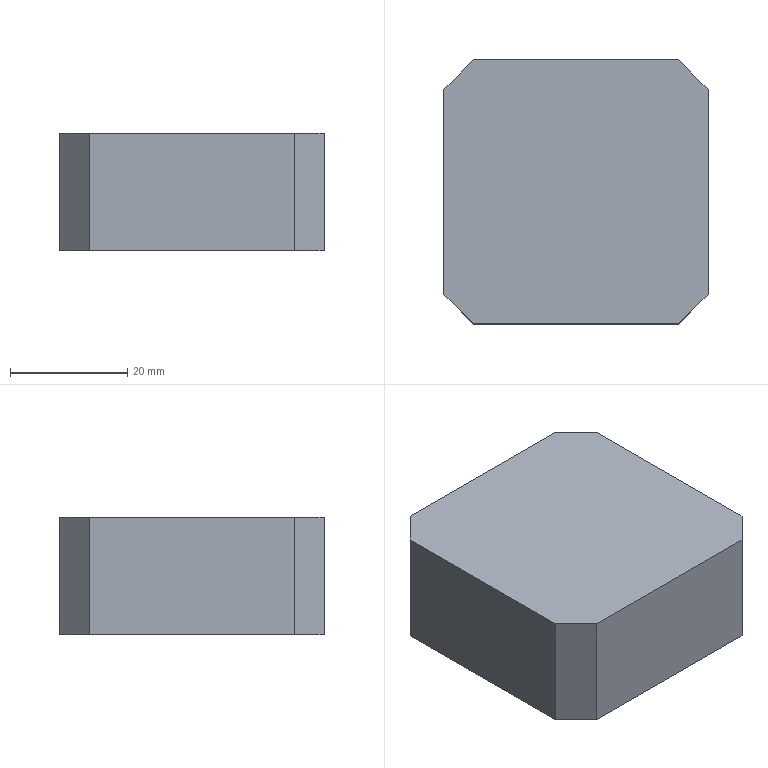Part | STEP file | 2012-06-08-019 | 1 solid | 10 faces | box 45 x 45 x 20 mm | volume 39500 mm3 | plane 10
STEP:
#1=CARTESIAN_POINT('',(0.,0.,0.));
#2=DIRECTION('',(0.,0.,1.));
#3=DIRECTION('',(1.,0.,0.));
#4=AXIS2_PLACEMENT_3D('',#1,#2,#3);
#5=CARTESIAN_POINT('',(22.5,-17.5,20.));
#6=VERTEX_POINT('',#5);
#7=CARTESIAN_POINT('',(22.5,17.5,20.));
#8=VERTEX_POINT('',#7);
#9=CARTESIAN_POINT('',(22.5,22.5,20.));
#10=DIRECTION('',(0.,1.,0.));
#11=VECTOR('',#10,1.);
#12=LINE('',#9,#11);
#13=CARTESIAN_POINT('',(22.5,22.5,20.));
#14=DIRECTION('',(-1.,0.,0.));
#15=DIRECTION('',(0.,-1.,0.));
#16=AXIS2_PLACEMENT_3D('',#13,#14,#15);
#17=PLANE('',#16);
#18=CARTESIAN_POINT('',(0.,0.));
#19=DIRECTION('',(-1.,0.));
#20=VECTOR('',#19,1.);
#21=LINE('',#18,#20);
#22=(GEOMETRIC_REPRESENTATION_CONTEXT(2)PARAMETRIC_REPRESENTATION_CONTEXT()REPRESENTATION_CONTEXT('',''));
#23=DEFINITIONAL_REPRESENTATION('',(#21),#22);
#24=PCURVE('',#17,#23);
#25=CARTESIAN_POINT('',(22.5,-22.5,20.));
#26=DIRECTION('',(0.,0.,1.));
#27=DIRECTION('',(1.,0.,0.));
#28=AXIS2_PLACEMENT_3D('',#25,#26,#27);
#29=PLANE('',#28);
#30=CARTESIAN_POINT('',(0.,45.));
#31=DIRECTION('',(0.,1.));
#32=VECTOR('',#31,1.);
#33=LINE('',#30,#32);
#34=(GEOMETRIC_REPRESENTATION_CONTEXT(2)PARAMETRIC_REPRESENTATION_CONTEXT()REPRESENTATION_CONTEXT('',''));
#35=DEFINITIONAL_REPRESENTATION('',(#33),#34);
#36=PCURVE('',#29,#35);
#37=SURFACE_CURVE('',#12,(#24,#36),.PCURVE_S1.);
#38=EDGE_CURVE('',#6,#8,#37,.T.);
#39=ORIENTED_EDGE('',*,*,#38,.F.);
#40=CARTESIAN_POINT('',(22.5,-17.5,0.));
#41=VERTEX_POINT('',#40);
#42=CARTESIAN_POINT('',(22.5,-17.5,20.));
#43=DIRECTION('',(0.,0.,-1.));
#44=VECTOR('',#43,1.);
#45=LINE('',#42,#44);
#46=CARTESIAN_POINT('',(40.,0.));
#47=DIRECTION('',(0.,-1.));
#48=VECTOR('',#47,1.);
#49=LINE('',#46,#48);
#50=(GEOMETRIC_REPRESENTATION_CONTEXT(2)PARAMETRIC_REPRESENTATION_CONTEXT()REPRESENTATION_CONTEXT('',''));
#51=DEFINITIONAL_REPRESENTATION('',(#49),#50);
#52=PCURVE('',#17,#51);
#53=CARTESIAN_POINT('',(22.5,-17.5,20.));
#54=DIRECTION('',(-0.7071,0.7071,0.));
#55=DIRECTION('',(-0.7071,-0.7071,0.));
#56=AXIS2_PLACEMENT_3D('',#53,#54,#55);
#57=PLANE('',#56);
#58=CARTESIAN_POINT('',(0.,0.));
#59=DIRECTION('',(0.,-1.));
#60=VECTOR('',#59,1.);
#61=LINE('',#58,#60);
#62=(GEOMETRIC_REPRESENTATION_CONTEXT(2)PARAMETRIC_REPRESENTATION_CONTEXT()REPRESENTATION_CONTEXT('',''));
#63=DEFINITIONAL_REPRESENTATION('',(#61),#62);
#64=PCURVE('',#57,#63);
#65=SURFACE_CURVE('',#45,(#52,#64),.PCURVE_S1.);
#66=EDGE_CURVE('',#6,#41,#65,.T.);
#67=ORIENTED_EDGE('',*,*,#66,.T.);
#68=CARTESIAN_POINT('',(22.5,17.5,0.));
#69=VERTEX_POINT('',#68);
#70=CARTESIAN_POINT('',(22.5,22.5,0.));
#71=DIRECTION('',(0.,1.,0.));
#72=VECTOR('',#71,1.);
#73=LINE('',#70,#72);
#74=CARTESIAN_POINT('',(0.,-20.));
#75=DIRECTION('',(-1.,0.));
#76=VECTOR('',#75,1.);
#77=LINE('',#74,#76);
#78=(GEOMETRIC_REPRESENTATION_CONTEXT(2)PARAMETRIC_REPRESENTATION_CONTEXT()REPRESENTATION_CONTEXT('',''));
#79=DEFINITIONAL_REPRESENTATION('',(#77),#78);
#80=PCURVE('',#17,#79);
#81=CARTESIAN_POINT('',(22.5,-22.5,0.));
#82=DIRECTION('',(0.,0.,1.));
#83=DIRECTION('',(1.,0.,0.));
#84=AXIS2_PLACEMENT_3D('',#81,#82,#83);
#85=PLANE('',#84);
#86=CARTESIAN_POINT('',(0.,45.));
#87=DIRECTION('',(0.,1.));
#88=VECTOR('',#87,1.);
#89=LINE('',#86,#88);
#90=(GEOMETRIC_REPRESENTATION_CONTEXT(2)PARAMETRIC_REPRESENTATION_CONTEXT()REPRESENTATION_CONTEXT('',''));
#91=DEFINITIONAL_REPRESENTATION('',(#89),#90);
#92=PCURVE('',#85,#91);
#93=SURFACE_CURVE('',#73,(#80,#92),.PCURVE_S1.);
#94=EDGE_CURVE('',#41,#69,#93,.T.);
#95=ORIENTED_EDGE('',*,*,#94,.T.);
#96=CARTESIAN_POINT('',(22.5,17.5,20.));
#97=DIRECTION('',(0.,0.,1.));
#98=VECTOR('',#97,1.);
#99=LINE('',#96,#98);
#100=CARTESIAN_POINT('',(5.,0.));
#101=DIRECTION('',(0.,1.));
#102=VECTOR('',#101,1.);
#103=LINE('',#100,#102);
#104=(GEOMETRIC_REPRESENTATION_CONTEXT(2)PARAMETRIC_REPRESENTATION_CONTEXT()REPRESENTATION_CONTEXT('',''));
#105=DEFINITIONAL_REPRESENTATION('',(#103),#104);
#106=PCURVE('',#17,#105);
#107=CARTESIAN_POINT('',(17.5,22.5,20.));
#108=DIRECTION('',(-0.7071,-0.7071,0.));
#109=DIRECTION('',(0.7071,-0.7071,0.));
#110=AXIS2_PLACEMENT_3D('',#107,#108,#109);
#111=PLANE('',#110);
#112=CARTESIAN_POINT('',(7.071,0.));
#113=DIRECTION('',(0.,1.));
#114=VECTOR('',#113,1.);
#115=LINE('',#112,#114);
#116=(GEOMETRIC_REPRESENTATION_CONTEXT(2)PARAMETRIC_REPRESENTATION_CONTEXT()REPRESENTATION_CONTEXT('',''));
#117=DEFINITIONAL_REPRESENTATION('',(#115),#116);
#118=PCURVE('',#111,#117);
#119=SURFACE_CURVE('',#99,(#106,#118),.PCURVE_S1.);
#120=EDGE_CURVE('',#69,#8,#119,.T.);
#121=ORIENTED_EDGE('',*,*,#120,.T.);
#122=EDGE_LOOP('',(#39,#67,#95,#121));
#123=FACE_BOUND('',#122,.T.);
#124=ADVANCED_FACE('',(#123),#17,.F.);
#125=CARTESIAN_POINT('',(17.5,22.5,0.));
#126=VERTEX_POINT('',#125);
#127=CARTESIAN_POINT('',(-17.5,22.5,0.));
#128=VERTEX_POINT('',#127);
#129=CARTESIAN_POINT('',(-22.5,22.5,0.));
#130=DIRECTION('',(-1.,0.,0.));
#131=VECTOR('',#130,1.);
#132=LINE('',#129,#131);
#133=CARTESIAN_POINT('',(-22.5,22.5,20.));
#134=DIRECTION('',(0.,-1.,0.));
#135=DIRECTION('',(0.,0.,-1.));
#136=AXIS2_PLACEMENT_3D('',#133,#134,#135);
#137=PLANE('',#136);
#138=CARTESIAN_POINT('',(20.,0.));
#139=DIRECTION('',(0.,-1.));
#140=VECTOR('',#139,1.);
#141=LINE('',#138,#140);
#142=(GEOMETRIC_REPRESENTATION_CONTEXT(2)PARAMETRIC_REPRESENTATION_CONTEXT()REPRESENTATION_CONTEXT('',''));
#143=DEFINITIONAL_REPRESENTATION('',(#141),#142);
#144=PCURVE('',#137,#143);
#145=CARTESIAN_POINT('',(-45.,45.));
#146=DIRECTION('',(-1.,0.));
#147=VECTOR('',#146,1.);
#148=LINE('',#145,#147);
#149=(GEOMETRIC_REPRESENTATION_CONTEXT(2)PARAMETRIC_REPRESENTATION_CONTEXT()REPRESENTATION_CONTEXT('',''));
#150=DEFINITIONAL_REPRESENTATION('',(#148),#149);
#151=PCURVE('',#85,#150);
#152=SURFACE_CURVE('',#132,(#144,#151),.PCURVE_S1.);
#153=EDGE_CURVE('',#126,#128,#152,.T.);
#154=ORIENTED_EDGE('',*,*,#153,.T.);
#155=CARTESIAN_POINT('',(-17.5,22.5,20.));
#156=VERTEX_POINT('',#155);
#157=CARTESIAN_POINT('',(-17.5,22.5,20.));
#158=DIRECTION('',(0.,0.,1.));
#159=VECTOR('',#158,1.);
#160=LINE('',#157,#159);
#161=CARTESIAN_POINT('',(0.,5.));
#162=DIRECTION('',(-1.,0.));
#163=VECTOR('',#162,1.);
#164=LINE('',#161,#163);
#165=(GEOMETRIC_REPRESENTATION_CONTEXT(2)PARAMETRIC_REPRESENTATION_CONTEXT()REPRESENTATION_CONTEXT('',''));
#166=DEFINITIONAL_REPRESENTATION('',(#164),#165);
#167=PCURVE('',#137,#166);
#168=CARTESIAN_POINT('',(-22.5,17.5,20.));
#169=DIRECTION('',(0.7071,-0.7071,0.));
#170=DIRECTION('',(0.7071,0.7071,0.));
#171=AXIS2_PLACEMENT_3D('',#168,#169,#170);
#172=PLANE('',#171);
#173=CARTESIAN_POINT('',(7.071,0.));
#174=DIRECTION('',(0.,1.));
#175=VECTOR('',#174,1.);
#176=LINE('',#173,#175);
#177=(GEOMETRIC_REPRESENTATION_CONTEXT(2)PARAMETRIC_REPRESENTATION_CONTEXT()REPRESENTATION_CONTEXT('',''));
#178=DEFINITIONAL_REPRESENTATION('',(#176),#177);
#179=PCURVE('',#172,#178);
#180=SURFACE_CURVE('',#160,(#167,#179),.PCURVE_S1.);
#181=EDGE_CURVE('',#128,#156,#180,.T.);
#182=ORIENTED_EDGE('',*,*,#181,.T.);
#183=CARTESIAN_POINT('',(17.5,22.5,20.));
#184=VERTEX_POINT('',#183);
#185=CARTESIAN_POINT('',(-22.5,22.5,20.));
#186=DIRECTION('',(-1.,0.,0.));
#187=VECTOR('',#186,1.);
#188=LINE('',#185,#187);
#189=CARTESIAN_POINT('',(0.,0.));
#190=DIRECTION('',(0.,-1.));
#191=VECTOR('',#190,1.);
#192=LINE('',#189,#191);
#193=(GEOMETRIC_REPRESENTATION_CONTEXT(2)PARAMETRIC_REPRESENTATION_CONTEXT()REPRESENTATION_CONTEXT('',''));
#194=DEFINITIONAL_REPRESENTATION('',(#192),#193);
#195=PCURVE('',#137,#194);
#196=CARTESIAN_POINT('',(-45.,45.));
#197=DIRECTION('',(-1.,0.));
#198=VECTOR('',#197,1.);
#199=LINE('',#196,#198);
#200=(GEOMETRIC_REPRESENTATION_CONTEXT(2)PARAMETRIC_REPRESENTATION_CONTEXT()REPRESENTATION_CONTEXT('',''));
#201=DEFINITIONAL_REPRESENTATION('',(#199),#200);
#202=PCURVE('',#29,#201);
#203=SURFACE_CURVE('',#188,(#195,#202),.PCURVE_S1.);
#204=EDGE_CURVE('',#184,#156,#203,.T.);
#205=ORIENTED_EDGE('',*,*,#204,.F.);
#206=CARTESIAN_POINT('',(17.5,22.5,20.));
#207=DIRECTION('',(0.,0.,-1.));
#208=VECTOR('',#207,1.);
#209=LINE('',#206,#208);
#210=CARTESIAN_POINT('',(0.,40.));
#211=DIRECTION('',(1.,0.));
#212=VECTOR('',#211,1.);
#213=LINE('',#210,#212);
#214=(GEOMETRIC_REPRESENTATION_CONTEXT(2)PARAMETRIC_REPRESENTATION_CONTEXT()REPRESENTATION_CONTEXT('',''));
#215=DEFINITIONAL_REPRESENTATION('',(#213),#214);
#216=PCURVE('',#137,#215);
#217=CARTESIAN_POINT('',(0.,0.));
#218=DIRECTION('',(0.,-1.));
#219=VECTOR('',#218,1.);
#220=LINE('',#217,#219);
#221=(GEOMETRIC_REPRESENTATION_CONTEXT(2)PARAMETRIC_REPRESENTATION_CONTEXT()REPRESENTATION_CONTEXT('',''));
#222=DEFINITIONAL_REPRESENTATION('',(#220),#221);
#223=PCURVE('',#111,#222);
#224=SURFACE_CURVE('',#209,(#216,#223),.PCURVE_S1.);
#225=EDGE_CURVE('',#184,#126,#224,.T.);
#226=ORIENTED_EDGE('',*,*,#225,.T.);
#227=EDGE_LOOP('',(#154,#182,#205,#226));
#228=FACE_BOUND('',#227,.T.);
#229=ADVANCED_FACE('',(#228),#137,.F.);
#230=CARTESIAN_POINT('',(-22.5,17.5,0.));
#231=VERTEX_POINT('',#230);
#232=CARTESIAN_POINT('',(-22.5,-17.5,0.));
#233=VERTEX_POINT('',#232);
#234=CARTESIAN_POINT('',(-22.5,22.5,0.));
#235=DIRECTION('',(0.,-1.,0.));
#236=VECTOR('',#235,1.);
#237=LINE('',#234,#236);
#238=CARTESIAN_POINT('',(-22.5,22.5,20.));
#239=DIRECTION('',(1.,0.,0.));
#240=DIRECTION('',(0.,1.,0.));
#241=AXIS2_PLACEMENT_3D('',#238,#239,#240);
#242=PLANE('',#241);
#243=CARTESIAN_POINT('',(0.,-20.));
#244=DIRECTION('',(-1.,0.));
#245=VECTOR('',#244,1.);
#246=LINE('',#243,#245);
#247=(GEOMETRIC_REPRESENTATION_CONTEXT(2)PARAMETRIC_REPRESENTATION_CONTEXT()REPRESENTATION_CONTEXT('',''));
#248=DEFINITIONAL_REPRESENTATION('',(#246),#247);
#249=PCURVE('',#242,#248);
#250=CARTESIAN_POINT('',(-45.,45.));
#251=DIRECTION('',(0.,-1.));
#252=VECTOR('',#251,1.);
#253=LINE('',#250,#252);
#254=(GEOMETRIC_REPRESENTATION_CONTEXT(2)PARAMETRIC_REPRESENTATION_CONTEXT()REPRESENTATION_CONTEXT('',''));
#255=DEFINITIONAL_REPRESENTATION('',(#253),#254);
#256=PCURVE('',#85,#255);
#257=SURFACE_CURVE('',#237,(#249,#256),.PCURVE_S1.);
#258=EDGE_CURVE('',#231,#233,#257,.T.);
#259=ORIENTED_EDGE('',*,*,#258,.T.);
#260=CARTESIAN_POINT('',(-22.5,-17.5,20.));
#261=VERTEX_POINT('',#260);
#262=CARTESIAN_POINT('',(-22.5,-17.5,20.));
#263=DIRECTION('',(0.,0.,1.));
#264=VECTOR('',#263,1.);
#265=LINE('',#262,#264);
#266=CARTESIAN_POINT('',(-40.,0.));
#267=DIRECTION('',(0.,1.));
#268=VECTOR('',#267,1.);
#269=LINE('',#266,#268);
#270=(GEOMETRIC_REPRESENTATION_CONTEXT(2)PARAMETRIC_REPRESENTATION_CONTEXT()REPRESENTATION_CONTEXT('',''));
#271=DEFINITIONAL_REPRESENTATION('',(#269),#270);
#272=PCURVE('',#242,#271);
#273=CARTESIAN_POINT('',(-17.5,-22.5,20.));
#274=DIRECTION('',(0.7071,0.7071,0.));
#275=DIRECTION('',(-0.7071,0.7071,0.));
#276=AXIS2_PLACEMENT_3D('',#273,#274,#275);
#277=PLANE('',#276);
#278=CARTESIAN_POINT('',(7.071,0.));
#279=DIRECTION('',(0.,1.));
#280=VECTOR('',#279,1.);
#281=LINE('',#278,#280);
#282=(GEOMETRIC_REPRESENTATION_CONTEXT(2)PARAMETRIC_REPRESENTATION_CONTEXT()REPRESENTATION_CONTEXT('',''));
#283=DEFINITIONAL_REPRESENTATION('',(#281),#282);
#284=PCURVE('',#277,#283);
#285=SURFACE_CURVE('',#265,(#272,#284),.PCURVE_S1.);
#286=EDGE_CURVE('',#233,#261,#285,.T.);
#287=ORIENTED_EDGE('',*,*,#286,.T.);
#288=CARTESIAN_POINT('',(-22.5,17.5,20.));
#289=VERTEX_POINT('',#288);
#290=CARTESIAN_POINT('',(-22.5,22.5,20.));
#291=DIRECTION('',(0.,-1.,0.));
#292=VECTOR('',#291,1.);
#293=LINE('',#290,#292);
#294=CARTESIAN_POINT('',(0.,0.));
#295=DIRECTION('',(-1.,0.));
#296=VECTOR('',#295,1.);
#297=LINE('',#294,#296);
#298=(GEOMETRIC_REPRESENTATION_CONTEXT(2)PARAMETRIC_REPRESENTATION_CONTEXT()REPRESENTATION_CONTEXT('',''));
#299=DEFINITIONAL_REPRESENTATION('',(#297),#298);
#300=PCURVE('',#242,#299);
#301=CARTESIAN_POINT('',(-45.,45.));
#302=DIRECTION('',(0.,-1.));
#303=VECTOR('',#302,1.);
#304=LINE('',#301,#303);
#305=(GEOMETRIC_REPRESENTATION_CONTEXT(2)PARAMETRIC_REPRESENTATION_CONTEXT()REPRESENTATION_CONTEXT('',''));
#306=DEFINITIONAL_REPRESENTATION('',(#304),#305);
#307=PCURVE('',#29,#306);
#308=SURFACE_CURVE('',#293,(#300,#307),.PCURVE_S1.);
#309=EDGE_CURVE('',#289,#261,#308,.T.);
#310=ORIENTED_EDGE('',*,*,#309,.F.);
#311=CARTESIAN_POINT('',(-22.5,17.5,20.));
#312=DIRECTION('',(0.,0.,-1.));
#313=VECTOR('',#312,1.);
#314=LINE('',#311,#313);
#315=CARTESIAN_POINT('',(-5.,0.));
#316=DIRECTION('',(0.,-1.));
#317=VECTOR('',#316,1.);
#318=LINE('',#315,#317);
#319=(GEOMETRIC_REPRESENTATION_CONTEXT(2)PARAMETRIC_REPRESENTATION_CONTEXT()REPRESENTATION_CONTEXT('',''));
#320=DEFINITIONAL_REPRESENTATION('',(#318),#319);
#321=PCURVE('',#242,#320);
#322=CARTESIAN_POINT('',(0.,0.));
#323=DIRECTION('',(0.,-1.));
#324=VECTOR('',#323,1.);
#325=LINE('',#322,#324);
#326=(GEOMETRIC_REPRESENTATION_CONTEXT(2)PARAMETRIC_REPRESENTATION_CONTEXT()REPRESENTATION_CONTEXT('',''));
#327=DEFINITIONAL_REPRESENTATION('',(#325),#326);
#328=PCURVE('',#172,#327);
#329=SURFACE_CURVE('',#314,(#321,#328),.PCURVE_S1.);
#330=EDGE_CURVE('',#289,#231,#329,.T.);
#331=ORIENTED_EDGE('',*,*,#330,.T.);
#332=EDGE_LOOP('',(#259,#287,#310,#331));
#333=FACE_BOUND('',#332,.T.);
#334=ADVANCED_FACE('',(#333),#242,.F.);
#335=CARTESIAN_POINT('',(-17.5,-22.5,20.));
#336=VERTEX_POINT('',#335);
#337=CARTESIAN_POINT('',(17.5,-22.5,20.));
#338=VERTEX_POINT('',#337);
#339=CARTESIAN_POINT('',(-22.5,-22.5,20.));
#340=DIRECTION('',(1.,0.,0.));
#341=VECTOR('',#340,1.);
#342=LINE('',#339,#341);
#343=CARTESIAN_POINT('',(-22.5,-22.5,20.));
#344=DIRECTION('',(0.,1.,0.));
#345=DIRECTION('',(0.,0.,1.));
#346=AXIS2_PLACEMENT_3D('',#343,#344,#345);
#347=PLANE('',#346);
#348=CARTESIAN_POINT('',(0.,0.));
#349=DIRECTION('',(0.,1.));
#350=VECTOR('',#349,1.);
#351=LINE('',#348,#350);
#352=(GEOMETRIC_REPRESENTATION_CONTEXT(2)PARAMETRIC_REPRESENTATION_CONTEXT()REPRESENTATION_CONTEXT('',''));
#353=DEFINITIONAL_REPRESENTATION('',(#351),#352);
#354=PCURVE('',#347,#353);
#355=CARTESIAN_POINT('',(-45.,0.));
#356=DIRECTION('',(1.,0.));
#357=VECTOR('',#356,1.);
#358=LINE('',#355,#357);
#359=(GEOMETRIC_REPRESENTATION_CONTEXT(2)PARAMETRIC_REPRESENTATION_CONTEXT()REPRESENTATION_CONTEXT('',''));
#360=DEFINITIONAL_REPRESENTATION('',(#358),#359);
#361=PCURVE('',#29,#360);
#362=SURFACE_CURVE('',#342,(#354,#361),.PCURVE_S1.);
#363=EDGE_CURVE('',#336,#338,#362,.T.);
#364=ORIENTED_EDGE('',*,*,#363,.F.);
#365=CARTESIAN_POINT('',(-17.5,-22.5,0.));
#366=VERTEX_POINT('',#365);
#367=CARTESIAN_POINT('',(-17.5,-22.5,20.));
#368=DIRECTION('',(0.,0.,-1.));
#369=VECTOR('',#368,1.);
#370=LINE('',#367,#369);
#371=CARTESIAN_POINT('',(0.,5.));
#372=DIRECTION('',(-1.,0.));
#373=VECTOR('',#372,1.);
#374=LINE('',#371,#373);
#375=(GEOMETRIC_REPRESENTATION_CONTEXT(2)PARAMETRIC_REPRESENTATION_CONTEXT()REPRESENTATION_CONTEXT('',''));
#376=DEFINITIONAL_REPRESENTATION('',(#374),#375);
#377=PCURVE('',#347,#376);
#378=CARTESIAN_POINT('',(0.,0.));
#379=DIRECTION('',(0.,-1.));
#380=VECTOR('',#379,1.);
#381=LINE('',#378,#380);
#382=(GEOMETRIC_REPRESENTATION_CONTEXT(2)PARAMETRIC_REPRESENTATION_CONTEXT()REPRESENTATION_CONTEXT('',''));
#383=DEFINITIONAL_REPRESENTATION('',(#381),#382);
#384=PCURVE('',#277,#383);
#385=SURFACE_CURVE('',#370,(#377,#384),.PCURVE_S1.);
#386=EDGE_CURVE('',#336,#366,#385,.T.);
#387=ORIENTED_EDGE('',*,*,#386,.T.);
#388=CARTESIAN_POINT('',(17.5,-22.5,0.));
#389=VERTEX_POINT('',#388);
#390=CARTESIAN_POINT('',(-22.5,-22.5,0.));
#391=DIRECTION('',(1.,0.,0.));
#392=VECTOR('',#391,1.);
#393=LINE('',#390,#392);
#394=CARTESIAN_POINT('',(-20.,0.));
#395=DIRECTION('',(0.,1.));
#396=VECTOR('',#395,1.);
#397=LINE('',#394,#396);
#398=(GEOMETRIC_REPRESENTATION_CONTEXT(2)PARAMETRIC_REPRESENTATION_CONTEXT()REPRESENTATION_CONTEXT('',''));
#399=DEFINITIONAL_REPRESENTATION('',(#397),#398);
#400=PCURVE('',#347,#399);
#401=CARTESIAN_POINT('',(-45.,0.));
#402=DIRECTION('',(1.,0.));
#403=VECTOR('',#402,1.);
#404=LINE('',#401,#403);
#405=(GEOMETRIC_REPRESENTATION_CONTEXT(2)PARAMETRIC_REPRESENTATION_CONTEXT()REPRESENTATION_CONTEXT('',''));
#406=DEFINITIONAL_REPRESENTATION('',(#404),#405);
#407=PCURVE('',#85,#406);
#408=SURFACE_CURVE('',#393,(#400,#407),.PCURVE_S1.);
#409=EDGE_CURVE('',#366,#389,#408,.T.);
#410=ORIENTED_EDGE('',*,*,#409,.T.);
#411=CARTESIAN_POINT('',(17.5,-22.5,20.));
#412=DIRECTION('',(0.,0.,1.));
#413=VECTOR('',#412,1.);
#414=LINE('',#411,#413);
#415=CARTESIAN_POINT('',(0.,40.));
#416=DIRECTION('',(1.,0.));
#417=VECTOR('',#416,1.);
#418=LINE('',#415,#417);
#419=(GEOMETRIC_REPRESENTATION_CONTEXT(2)PARAMETRIC_REPRESENTATION_CONTEXT()REPRESENTATION_CONTEXT('',''));
#420=DEFINITIONAL_REPRESENTATION('',(#418),#419);
#421=PCURVE('',#347,#420);
#422=CARTESIAN_POINT('',(7.071,0.));
#423=DIRECTION('',(0.,1.));
#424=VECTOR('',#423,1.);
#425=LINE('',#422,#424);
#426=(GEOMETRIC_REPRESENTATION_CONTEXT(2)PARAMETRIC_REPRESENTATION_CONTEXT()REPRESENTATION_CONTEXT('',''));
#427=DEFINITIONAL_REPRESENTATION('',(#425),#426);
#428=PCURVE('',#57,#427);
#429=SURFACE_CURVE('',#414,(#421,#428),.PCURVE_S1.);
#430=EDGE_CURVE('',#389,#338,#429,.T.);
#431=ORIENTED_EDGE('',*,*,#430,.T.);
#432=EDGE_LOOP('',(#364,#387,#410,#431));
#433=FACE_BOUND('',#432,.T.);
#434=ADVANCED_FACE('',(#433),#347,.F.);
#435=ORIENTED_EDGE('',*,*,#309,.T.);
#436=CARTESIAN_POINT('',(2.5,-42.5,20.));
#437=DIRECTION('',(0.7071,-0.7071,0.));
#438=VECTOR('',#437,1.);
#439=LINE('',#436,#438);
#440=CARTESIAN_POINT('',(-20.,-20.));
#441=DIRECTION('',(0.7071,-0.7071));
#442=VECTOR('',#441,1.);
#443=LINE('',#440,#442);
#444=(GEOMETRIC_REPRESENTATION_CONTEXT(2)PARAMETRIC_REPRESENTATION_CONTEXT()REPRESENTATION_CONTEXT('',''));
#445=DEFINITIONAL_REPRESENTATION('',(#443),#444);
#446=PCURVE('',#29,#445);
#447=CARTESIAN_POINT('',(-28.284,0.));
#448=DIRECTION('',(-1.,0.));
#449=VECTOR('',#448,1.);
#450=LINE('',#447,#449);
#451=(GEOMETRIC_REPRESENTATION_CONTEXT(2)PARAMETRIC_REPRESENTATION_CONTEXT()REPRESENTATION_CONTEXT('',''));
#452=DEFINITIONAL_REPRESENTATION('',(#450),#451);
#453=PCURVE('',#277,#452);
#454=SURFACE_CURVE('',#439,(#446,#453),.PCURVE_S1.);
#455=EDGE_CURVE('',#261,#336,#454,.T.);
#456=ORIENTED_EDGE('',*,*,#455,.T.);
#457=ORIENTED_EDGE('',*,*,#363,.T.);
#458=CARTESIAN_POINT('',(20.,-20.,20.));
#459=DIRECTION('',(0.7071,0.7071,0.));
#460=VECTOR('',#459,1.);
#461=LINE('',#458,#460);
#462=CARTESIAN_POINT('',(-2.5,2.5));
#463=DIRECTION('',(0.7071,0.7071));
#464=VECTOR('',#463,1.);
#465=LINE('',#462,#464);
#466=(GEOMETRIC_REPRESENTATION_CONTEXT(2)PARAMETRIC_REPRESENTATION_CONTEXT()REPRESENTATION_CONTEXT('',''));
#467=DEFINITIONAL_REPRESENTATION('',(#465),#466);
#468=PCURVE('',#29,#467);
#469=CARTESIAN_POINT('',(3.536,0.));
#470=DIRECTION('',(-1.,0.));
#471=VECTOR('',#470,1.);
#472=LINE('',#469,#471);
#473=(GEOMETRIC_REPRESENTATION_CONTEXT(2)PARAMETRIC_REPRESENTATION_CONTEXT()REPRESENTATION_CONTEXT('',''));
#474=DEFINITIONAL_REPRESENTATION('',(#472),#473);
#475=PCURVE('',#57,#474);
#476=SURFACE_CURVE('',#461,(#468,#475),.PCURVE_S1.);
#477=EDGE_CURVE('',#338,#6,#476,.T.);
#478=ORIENTED_EDGE('',*,*,#477,.T.);
#479=ORIENTED_EDGE('',*,*,#38,.T.);
#480=CARTESIAN_POINT('',(42.5,-2.5,20.));
#481=DIRECTION('',(-0.7071,0.7071,0.));
#482=VECTOR('',#481,1.);
#483=LINE('',#480,#482);
#484=CARTESIAN_POINT('',(20.,20.));
#485=DIRECTION('',(-0.7071,0.7071));
#486=VECTOR('',#485,1.);
#487=LINE('',#484,#486);
#488=(GEOMETRIC_REPRESENTATION_CONTEXT(2)PARAMETRIC_REPRESENTATION_CONTEXT()REPRESENTATION_CONTEXT('',''));
#489=DEFINITIONAL_REPRESENTATION('',(#487),#488);
#490=PCURVE('',#29,#489);
#491=CARTESIAN_POINT('',(35.355,0.));
#492=DIRECTION('',(-1.,0.));
#493=VECTOR('',#492,1.);
#494=LINE('',#491,#493);
#495=(GEOMETRIC_REPRESENTATION_CONTEXT(2)PARAMETRIC_REPRESENTATION_CONTEXT()REPRESENTATION_CONTEXT('',''));
#496=DEFINITIONAL_REPRESENTATION('',(#494),#495);
#497=PCURVE('',#111,#496);
#498=SURFACE_CURVE('',#483,(#490,#497),.PCURVE_S1.);
#499=EDGE_CURVE('',#8,#184,#498,.T.);
#500=ORIENTED_EDGE('',*,*,#499,.T.);
#501=ORIENTED_EDGE('',*,*,#204,.T.);
#502=CARTESIAN_POINT('',(-20.,20.,20.));
#503=DIRECTION('',(-0.7071,-0.7071,0.));
#504=VECTOR('',#503,1.);
#505=LINE('',#502,#504);
#506=CARTESIAN_POINT('',(-42.5,42.5));
#507=DIRECTION('',(-0.7071,-0.7071));
#508=VECTOR('',#507,1.);
#509=LINE('',#506,#508);
#510=(GEOMETRIC_REPRESENTATION_CONTEXT(2)PARAMETRIC_REPRESENTATION_CONTEXT()REPRESENTATION_CONTEXT('',''));
#511=DEFINITIONAL_REPRESENTATION('',(#509),#510);
#512=PCURVE('',#29,#511);
#513=CARTESIAN_POINT('',(3.536,0.));
#514=DIRECTION('',(-1.,0.));
#515=VECTOR('',#514,1.);
#516=LINE('',#513,#515);
#517=(GEOMETRIC_REPRESENTATION_CONTEXT(2)PARAMETRIC_REPRESENTATION_CONTEXT()REPRESENTATION_CONTEXT('',''));
#518=DEFINITIONAL_REPRESENTATION('',(#516),#517);
#519=PCURVE('',#172,#518);
#520=SURFACE_CURVE('',#505,(#512,#519),.PCURVE_S1.);
#521=EDGE_CURVE('',#156,#289,#520,.T.);
#522=ORIENTED_EDGE('',*,*,#521,.T.);
#523=EDGE_LOOP('',(#435,#456,#457,#478,#479,#500,#501,#522));
#524=FACE_BOUND('',#523,.T.);
#525=ADVANCED_FACE('',(#524),#29,.T.);
#526=ORIENTED_EDGE('',*,*,#409,.F.);
#527=CARTESIAN_POINT('',(-17.5,-22.5,0.));
#528=DIRECTION('',(-0.7071,0.7071,0.));
#529=VECTOR('',#528,1.);
#530=LINE('',#527,#529);
#531=CARTESIAN_POINT('',(-40.,0.));
#532=DIRECTION('',(-0.7071,0.7071));
#533=VECTOR('',#532,1.);
#534=LINE('',#531,#533);
#535=(GEOMETRIC_REPRESENTATION_CONTEXT(2)PARAMETRIC_REPRESENTATION_CONTEXT()REPRESENTATION_CONTEXT('',''));
#536=DEFINITIONAL_REPRESENTATION('',(#534),#535);
#537=PCURVE('',#85,#536);
#538=CARTESIAN_POINT('',(0.,-20.));
#539=DIRECTION('',(1.,0.));
#540=VECTOR('',#539,1.);
#541=LINE('',#538,#540);
#542=(GEOMETRIC_REPRESENTATION_CONTEXT(2)PARAMETRIC_REPRESENTATION_CONTEXT()REPRESENTATION_CONTEXT('',''));
#543=DEFINITIONAL_REPRESENTATION('',(#541),#542);
#544=PCURVE('',#277,#543);
#545=SURFACE_CURVE('',#530,(#537,#544),.PCURVE_S1.);
#546=EDGE_CURVE('',#366,#233,#545,.T.);
#547=ORIENTED_EDGE('',*,*,#546,.T.);
#548=ORIENTED_EDGE('',*,*,#258,.F.);
#549=CARTESIAN_POINT('',(-22.5,17.5,0.));
#550=DIRECTION('',(0.7071,0.7071,0.));
#551=VECTOR('',#550,1.);
#552=LINE('',#549,#551);
#553=CARTESIAN_POINT('',(-45.,40.));
#554=DIRECTION('',(0.7071,0.7071));
#555=VECTOR('',#554,1.);
#556=LINE('',#553,#555);
#557=(GEOMETRIC_REPRESENTATION_CONTEXT(2)PARAMETRIC_REPRESENTATION_CONTEXT()REPRESENTATION_CONTEXT('',''));
#558=DEFINITIONAL_REPRESENTATION('',(#556),#557);
#559=PCURVE('',#85,#558);
#560=CARTESIAN_POINT('',(0.,-20.));
#561=DIRECTION('',(1.,0.));
#562=VECTOR('',#561,1.);
#563=LINE('',#560,#562);
#564=(GEOMETRIC_REPRESENTATION_CONTEXT(2)PARAMETRIC_REPRESENTATION_CONTEXT()REPRESENTATION_CONTEXT('',''));
#565=DEFINITIONAL_REPRESENTATION('',(#563),#564);
#566=PCURVE('',#172,#565);
#567=SURFACE_CURVE('',#552,(#559,#566),.PCURVE_S1.);
#568=EDGE_CURVE('',#231,#128,#567,.T.);
#569=ORIENTED_EDGE('',*,*,#568,.T.);
#570=ORIENTED_EDGE('',*,*,#153,.F.);
#571=CARTESIAN_POINT('',(17.5,22.5,0.));
#572=DIRECTION('',(0.7071,-0.7071,0.));
#573=VECTOR('',#572,1.);
#574=LINE('',#571,#573);
#575=CARTESIAN_POINT('',(-5.,45.));
#576=DIRECTION('',(0.7071,-0.7071));
#577=VECTOR('',#576,1.);
#578=LINE('',#575,#577);
#579=(GEOMETRIC_REPRESENTATION_CONTEXT(2)PARAMETRIC_REPRESENTATION_CONTEXT()REPRESENTATION_CONTEXT('',''));
#580=DEFINITIONAL_REPRESENTATION('',(#578),#579);
#581=PCURVE('',#85,#580);
#582=CARTESIAN_POINT('',(0.,-20.));
#583=DIRECTION('',(1.,0.));
#584=VECTOR('',#583,1.);
#585=LINE('',#582,#584);
#586=(GEOMETRIC_REPRESENTATION_CONTEXT(2)PARAMETRIC_REPRESENTATION_CONTEXT()REPRESENTATION_CONTEXT('',''));
#587=DEFINITIONAL_REPRESENTATION('',(#585),#586);
#588=PCURVE('',#111,#587);
#589=SURFACE_CURVE('',#574,(#581,#588),.PCURVE_S1.);
#590=EDGE_CURVE('',#126,#69,#589,.T.);
#591=ORIENTED_EDGE('',*,*,#590,.T.);
#592=ORIENTED_EDGE('',*,*,#94,.F.);
#593=CARTESIAN_POINT('',(22.5,-17.5,0.));
#594=DIRECTION('',(-0.7071,-0.7071,0.));
#595=VECTOR('',#594,1.);
#596=LINE('',#593,#595);
#597=CARTESIAN_POINT('',(0.,5.));
#598=DIRECTION('',(-0.7071,-0.7071));
#599=VECTOR('',#598,1.);
#600=LINE('',#597,#599);
#601=(GEOMETRIC_REPRESENTATION_CONTEXT(2)PARAMETRIC_REPRESENTATION_CONTEXT()REPRESENTATION_CONTEXT('',''));
#602=DEFINITIONAL_REPRESENTATION('',(#600),#601);
#603=PCURVE('',#85,#602);
#604=CARTESIAN_POINT('',(0.,-20.));
#605=DIRECTION('',(1.,0.));
#606=VECTOR('',#605,1.);
#607=LINE('',#604,#606);
#608=(GEOMETRIC_REPRESENTATION_CONTEXT(2)PARAMETRIC_REPRESENTATION_CONTEXT()REPRESENTATION_CONTEXT('',''));
#609=DEFINITIONAL_REPRESENTATION('',(#607),#608);
#610=PCURVE('',#57,#609);
#611=SURFACE_CURVE('',#596,(#603,#610),.PCURVE_S1.);
#612=EDGE_CURVE('',#41,#389,#611,.T.);
#613=ORIENTED_EDGE('',*,*,#612,.T.);
#614=EDGE_LOOP('',(#526,#547,#548,#569,#570,#591,#592,#613));
#615=FACE_BOUND('',#614,.T.);
#616=ADVANCED_FACE('',(#615),#85,.F.);
#617=ORIENTED_EDGE('',*,*,#455,.F.);
#618=ORIENTED_EDGE('',*,*,#286,.F.);
#619=ORIENTED_EDGE('',*,*,#546,.F.);
#620=ORIENTED_EDGE('',*,*,#386,.F.);
#621=EDGE_LOOP('',(#617,#618,#619,#620));
#622=FACE_BOUND('',#621,.T.);
#623=ADVANCED_FACE('',(#622),#277,.F.);
#624=ORIENTED_EDGE('',*,*,#477,.F.);
#625=ORIENTED_EDGE('',*,*,#430,.F.);
#626=ORIENTED_EDGE('',*,*,#612,.F.);
#627=ORIENTED_EDGE('',*,*,#66,.F.);
#628=EDGE_LOOP('',(#624,#625,#626,#627));
#629=FACE_BOUND('',#628,.T.);
#630=ADVANCED_FACE('',(#629),#57,.F.);
#631=ORIENTED_EDGE('',*,*,#521,.F.);
#632=ORIENTED_EDGE('',*,*,#181,.F.);
#633=ORIENTED_EDGE('',*,*,#568,.F.);
#634=ORIENTED_EDGE('',*,*,#330,.F.);
#635=EDGE_LOOP('',(#631,#632,#633,#634));
#636=FACE_BOUND('',#635,.T.);
#637=ADVANCED_FACE('',(#636),#172,.F.);
#638=ORIENTED_EDGE('',*,*,#499,.F.);
#639=ORIENTED_EDGE('',*,*,#120,.F.);
#640=ORIENTED_EDGE('',*,*,#590,.F.);
#641=ORIENTED_EDGE('',*,*,#225,.F.);
#642=EDGE_LOOP('',(#638,#639,#640,#641));
#643=FACE_BOUND('',#642,.T.);
#644=ADVANCED_FACE('',(#643),#111,.F.);
#645=CLOSED_SHELL('',(#124,#229,#334,#434,#525,#616,#623,#630,#637,#644));
#646=MANIFOLD_SOLID_BREP('',#645);
#647=(LENGTH_UNIT()NAMED_UNIT(*)SI_UNIT(.MILLI.,.METRE.));
#648=UNCERTAINTY_MEASURE_WITH_UNIT(LENGTH_MEASURE(0.0000001),#647,'','');
#649=(NAMED_UNIT(*)PLANE_ANGLE_UNIT()SI_UNIT($,.RADIAN.));
#650=(NAMED_UNIT(*)SI_UNIT($,.STERADIAN.)SOLID_ANGLE_UNIT());
#651=(GEOMETRIC_REPRESENTATION_CONTEXT(3)GLOBAL_UNCERTAINTY_ASSIGNED_CONTEXT((#648))GLOBAL_UNIT_ASSIGNED_CONTEXT((#647,#649,#650))REPRESENTATION_CONTEXT('',''));
#652=ADVANCED_BREP_SHAPE_REPRESENTATION('',(#4,#646),#651);